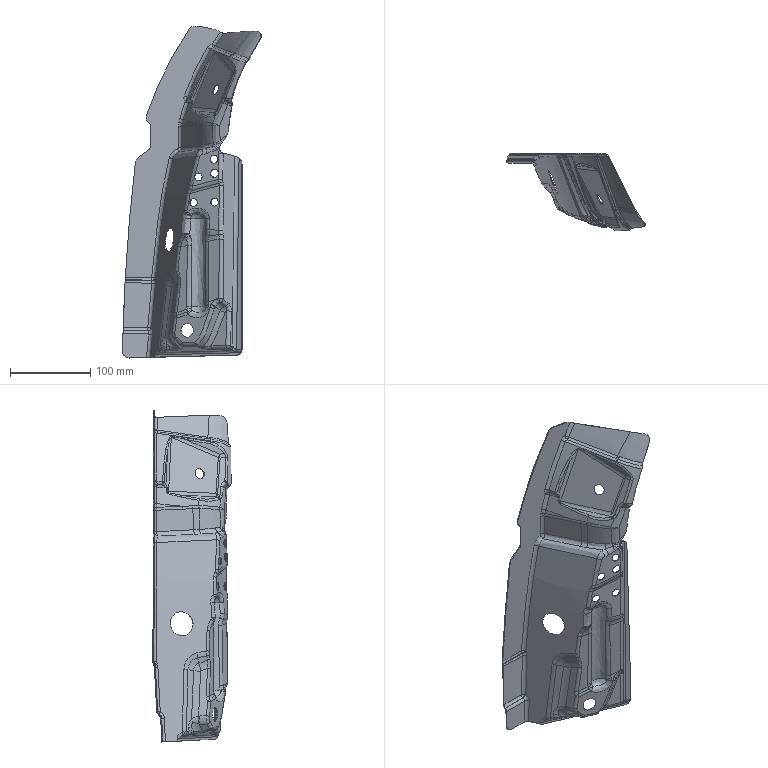Part | STEP file | FNA5401952 | 1 solid | 572 faces | box 172.44 x 97.142 x 412.618 mm | volume 89777 mm3 | spline 404 | cylinder 99 | plane 45 | sphere 14 | other 10 | commonest cylinder face diameters 10 x27 7.6 x11 12.4 x7 21.4 x6 23.8 x6 12 x5